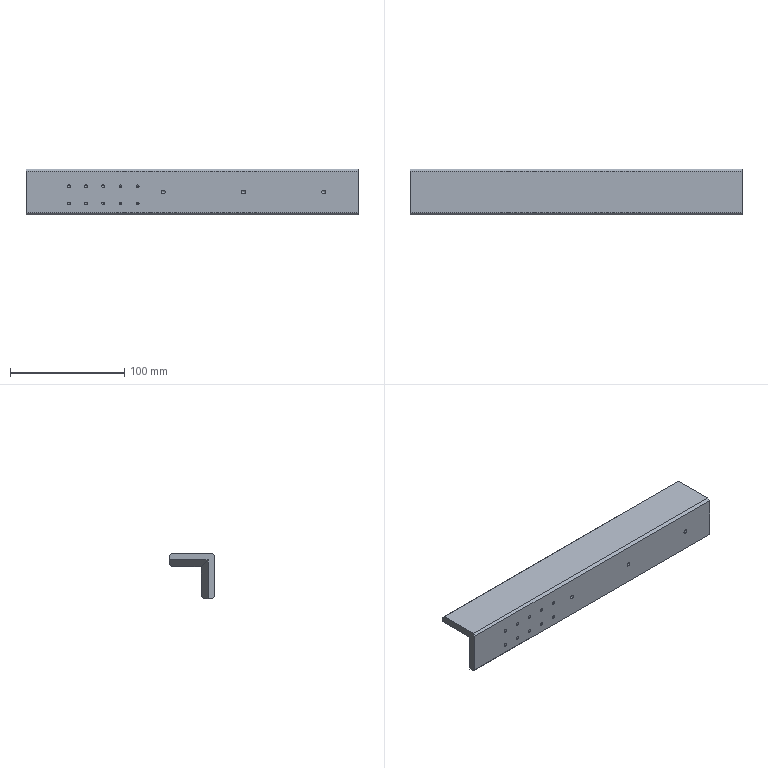CAM job | NX | 3+2 milling, drilling | part box 290 x 40 x 40 mm | stock box 295 x 45 x 45 mm
Tools:
number,name,description,diameter,corner_radius,flute_length,length,flutes
9,D10,平底铣刀-粗,10.0,0.0,35.0,75.0,2
10,D10-J,平底铣刀-精,10.0,0.0,35.0,75.0,2
1,D80R0.8飞刀,圆鼻刀-粗,80.0,0.8,50.0,75.0,2
1,D80R0.8飞刀-J,圆鼻刀-精,80.0,0.8,50.0,75.0,2
2,D6倒角刀,倒角刀,6.0,0.0,3.0,25.0,2
20,M3X0.5,丝锥,2.5,0.0,35.0,50.0,2
21,M4X0.7,丝锥,3.3,0.0,35.0,50.0,2
12,ZT2.5,钻头,2.5,0.0,35.0,50.0,2
13,钻头3.3,Twist Drill 3.3 mm,3.3,0.0,35.0,35.008,2
Operations:
program,operation,operation_type,tool,method,geometry_group,spindle_rpm,surface_speed,feed_per_tooth,feed_cut,feed_plunge,cut_length_mm,path_length_mm,cut_time_min,machine_time_min
B,底壁铣飞面一刀开粗_COPY,VolumeBased25DMillingOperation,D80R0.8飞刀,分层开粗-切深K-步距G,W-B,2800.0,703.696,0.5357,3000.0,100.0,3583.746,6935.966,1.195,1.53
B,底壁铣飞面一刀精光_COPY,VolumeBased25DMillingOperation,D80R0.8飞刀-J,侧刃精光-切深K-步距G,W-B,4000.0,1005.28,0.125,1000.0,100.0,397.998,433.998,0.398,0.4016
B,型腔铣开粗-中_COPY,CavityMilling,D10,分层开粗-切深K-步距G,W-B,8000.0,251.32,0.25,4000.0,100.0,76784.199,78243.745,19.196,19.418
B,型腔铣开粗-中_COPY_COPY,CavityMilling,D10,分层开粗-切深K-步距G,W-B,8000.0,251.32,0.25,4000.0,100.0,1180.651,1487.894,0.2952,0.3367
B,等高精光往复爬面_COPY_COPY,ZLevelMilling,D10,等高爬面-切深K-步距G,W-B,7000.0,219.911,0.3214,4500.0,100.0,4394.171,4424.812,0.9765,0.9795
B,平面去毛刺6X45L_COPY,SurfaceContour,D6倒角刀,爬面_倒角-切深0-步距G,W-B,6500.0,122.519,0.1154,1500.0,100.0,82.783,511.916,0.0552,0.0981
B,底壁铣倒角_COPY_1,VolumeBased25DMillingOperation,D6倒角刀,爬面_倒角-切深0-步距G,W-B,6500.0,122.522,0.0769,1000.0,100.0,594.32,696.327,0.5943,0.6045
B,C0.3封闭铣廓倒角6X45L_COPY,PlanarMilling,D6倒角刀,爬面_倒角-切深0-步距G,W-B,7000.0,131.0,0.0714,1000.0,100.0,300.0,396.2,0.3,0.3096
B,底壁铣精光底面-中_COPY,VolumeBased25DMillingOperation,D10-J,精光步距切深关,W-B,7000.0,175.0,0.0536,1500.0,100.0,1766.804,1848.804,1.178,1.186
B,等高精光-中_COPY,ZLevelMilling,D10-J,侧刃精光-切深K-步距G,W-B,8000.0,251.32,0.0625,1000.0,100.0,602.259,1016.527,0.6023,0.6437
B,等高精光往复爬面_COPY_1,ZLevelMilling,D10-J,等高爬面-切深K-步距G,W-B,7000.0,219.911,0.25,3500.0,100.0,22613.385,22703.893,6.461,6.47
A,顶面,FaceMilling,D80R0.8飞刀,侧刃精光-切深K-步距G,W-A,4000.0,1005.31,0.125,1000.0,100.0,384.0,420.0,0.384,0.3876
A,外形粗_2,VolumeBased25DMillingOperation,D10,METHOD,W-A,8000.0,251.327,0.3125,5000.0,80.0,35987.824,36066.624,7.198,7.205
A,等高精光往复爬面_COPY,ZLevelMilling,D10,等高爬面-切深K-步距G,W-A,7000.0,219.911,0.3214,4500.0,100.0,8788.34,8884.024,1.953,1.962
A,打点-深0.8,Operation,D6倒角刀,NONE,W-A,8000.0,150.796,0.0312,500.0,90.0,23.4,398.756,0.0468,0.0843
A,盲锥孔-M3螺纹底孔,Operation,ZT2.5,NONE,W-A,3000.0,23.562,0.0167,100.0,90.0,110.0,404.3,1.1,1.129
A,盲锥孔-M4螺纹底孔,Operation,钻头3.3,NONE,W-A,3000.0,31.102,0.02,120.0,90.0,36.274,254.563,0.3023,0.3241
A,仅选体,SurfaceContour,D6倒角刀,METHOD,W-A,8000.0,150.796,0.1875,3000.0,100.0,91.631,452.307,0.0305,0.0666
A,底壁铣倒角_COPY,VolumeBased25DMillingOperation,D6倒角刀,爬面_倒角-切深0-步距G,W-A,6500.0,122.522,0.0769,1000.0,100.0,603.03,730.862,0.603,0.6158
A,钻倒角_1,Operation,D6倒角刀,METHOD,W-A,8000.0,150.796,0.0312,500.0,0.0,47.5,299.673,0.095,0.1202
A,钻倒角_2,Operation,D6倒角刀,METHOD,W-A,8000.0,150.796,0.0312,500.0,0.0,15.6,217.328,0.0312,0.0514
A,盲锥孔-攻牙M3,Operation,M3X0.5,METHOD,W-A,1000.0,7.854,0.0003,0.5,90.0,80.0,344.3,160.0,160.026
A,盲锥孔-攻牙M4,Operation,M4X0.7,METHOD,W-A,800.0,8.294,0.0004,0.7,90.0,27.3,236.614,39.0,39.021
A,外形半精_2,VolumeBased25DMillingOperation,D10-J,METHOD,W-A,8000.0,251.327,0.0625,1000.0,100.0,2089.122,2372.351,2.089,2.117